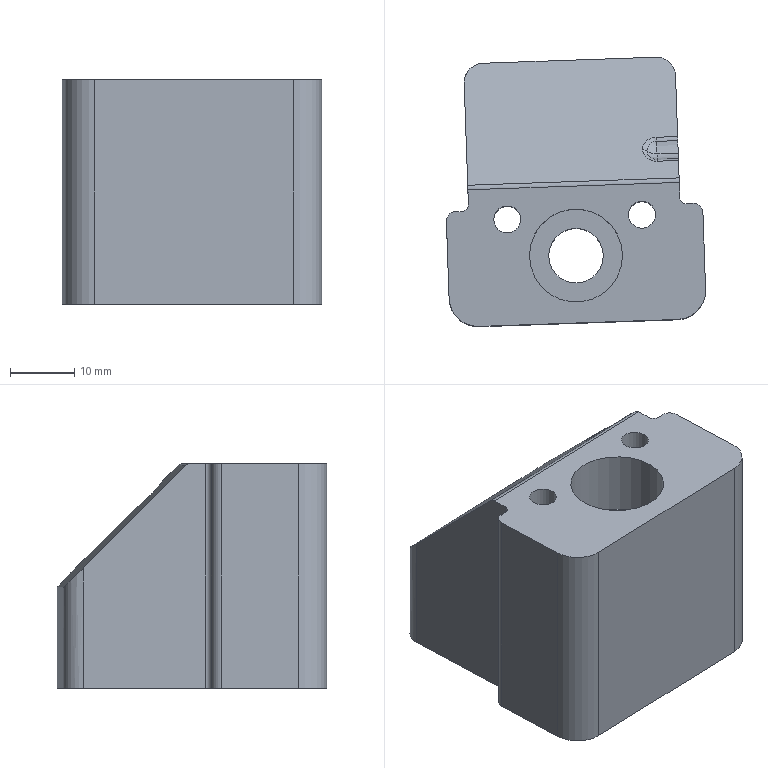Part | NX | features DIE-68 2 | 1 solid | 33 faces | box 40.398 x 41.991 x 35 mm | volume 41184 mm3 | cylinder 14 | plane 12 | spline 7 | commonest cylinder face diameters 2 x4 3 x2 4.201 x2 6 x2 9 x2 8.506 x1